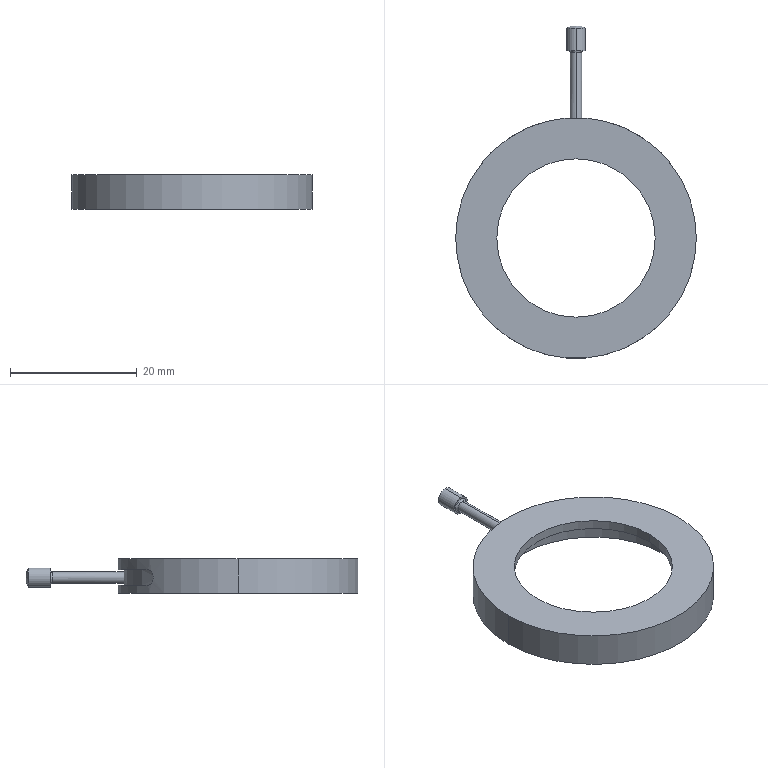Part | SolidWorks | features BaseBody 2 | 2 solids | 33 faces | box 38 x 52.6 x 5.5 mm | volume 2350 mm3 | cylinder 17 | plane 9 | spline 5 | cone 2 | commonest cylinder face diameters 1.6 x4 1 x2 1.8 x2 3 x2 25 x2 31.6 x2
STEP:
#1=CARTESIAN_POINT('',(12.618,14.205,1.7));
#2=VERTEX_POINT('',#1);
#3=CARTESIAN_POINT('',(-12.618,14.205,1.7));
#4=VERTEX_POINT('',#3);
#5=CARTESIAN_POINT('',(0.,0.,1.7));
#6=DIRECTION('',(0.,0.,1.));
#7=DIRECTION('',(-1.,0.,0.));
#8=AXIS2_PLACEMENT_3D('',#5,#6,#7);
#9=CIRCLE('',#8,19.);
#10=EDGE_CURVE('',#2,#4,#9,.T.);
#11=ORIENTED_EDGE('',*,*,#10,.T.);
#12=CARTESIAN_POINT('',(-12.618,14.205,-0.7));
#13=VERTEX_POINT('',#12);
#14=CARTESIAN_POINT('',(-12.618,14.205,1.7));
#15=CARTESIAN_POINT('',(-12.737,14.1,1.7));
#16=CARTESIAN_POINT('',(-12.852,13.995,1.669));
#17=CARTESIAN_POINT('',(-13.064,13.797,1.548));
#18=CARTESIAN_POINT('',(-13.16,13.705,1.459));
#19=CARTESIAN_POINT('',(-13.319,13.55,1.238));
#20=CARTESIAN_POINT('',(-13.383,13.487,1.104));
#21=CARTESIAN_POINT('',(-13.467,13.403,0.815));
#22=CARTESIAN_POINT('',(-13.49,13.38,0.657));
#23=CARTESIAN_POINT('',(-13.49,13.38,0.3439));
#24=CARTESIAN_POINT('',(-13.468,13.402,0.1866));
#25=CARTESIAN_POINT('',(-13.383,13.487,-0.1038));
#26=CARTESIAN_POINT('',(-13.32,13.549,-0.2361));
#27=CARTESIAN_POINT('',(-13.16,13.705,-0.4599));
#28=CARTESIAN_POINT('',(-13.065,13.796,-0.5481));
#29=CARTESIAN_POINT('',(-12.852,13.995,-0.6687));
#30=CARTESIAN_POINT('',(-12.737,14.1,-0.6996));
#31=CARTESIAN_POINT('',(-12.618,14.205,-0.7));
#32=B_SPLINE_CURVE_WITH_KNOTS('',3,(#14,#15,#16,#17,#18,#19,#20,#21,#22,#23,#24,#25,#26,#27,#28,#29,#30,#31),.UNSPECIFIED.,.F.,.F.,(4,2,2,2,2,2,2,2,4),(0.,0.0004687,0.0009374,0.001406,0.001875,0.002343,0.002812,0.003281,0.00375),.UNSPECIFIED.);
#33=EDGE_CURVE('',#4,#13,#32,.T.);
#34=ORIENTED_EDGE('',*,*,#33,.T.);
#35=CARTESIAN_POINT('',(12.618,14.205,-0.7));
#36=VERTEX_POINT('',#35);
#37=CARTESIAN_POINT('',(0.,0.,-0.7));
#38=DIRECTION('',(0.,0.,-1.));
#39=DIRECTION('',(-1.,0.,0.));
#40=AXIS2_PLACEMENT_3D('',#37,#38,#39);
#41=CIRCLE('',#40,19.);
#42=EDGE_CURVE('',#13,#36,#41,.T.);
#43=ORIENTED_EDGE('',*,*,#42,.T.);
#44=CARTESIAN_POINT('',(12.618,14.205,-0.7));
#45=CARTESIAN_POINT('',(12.737,14.1,-0.6996));
#46=CARTESIAN_POINT('',(12.852,13.995,-0.6689));
#47=CARTESIAN_POINT('',(13.064,13.797,-0.5484));
#48=CARTESIAN_POINT('',(13.16,13.705,-0.4594));
#49=CARTESIAN_POINT('',(13.319,13.55,-0.2378));
#50=CARTESIAN_POINT('',(13.383,13.487,-0.1039));
#51=CARTESIAN_POINT('',(13.467,13.403,0.185));
#52=CARTESIAN_POINT('',(13.49,13.38,0.343));
#53=CARTESIAN_POINT('',(13.49,13.38,0.6561));
#54=CARTESIAN_POINT('',(13.468,13.402,0.8134));
#55=CARTESIAN_POINT('',(13.383,13.487,1.104));
#56=CARTESIAN_POINT('',(13.32,13.549,1.236));
#57=CARTESIAN_POINT('',(13.16,13.705,1.46));
#58=CARTESIAN_POINT('',(13.065,13.796,1.548));
#59=CARTESIAN_POINT('',(12.852,13.995,1.669));
#60=CARTESIAN_POINT('',(12.737,14.1,1.7));
#61=CARTESIAN_POINT('',(12.618,14.205,1.7));
#62=B_SPLINE_CURVE_WITH_KNOTS('',3,(#44,#45,#46,#47,#48,#49,#50,#51,#52,#53,#54,#55,#56,#57,#58,#59,#60,#61),.UNSPECIFIED.,.F.,.F.,(4,2,2,2,2,2,2,2,4),(0.,0.0004687,0.0009374,0.001406,0.001875,0.002343,0.002812,0.003281,0.00375),.UNSPECIFIED.);
#63=EDGE_CURVE('',#36,#2,#62,.T.);
#64=ORIENTED_EDGE('',*,*,#63,.T.);
#65=EDGE_LOOP('',(#11,#34,#43,#64));
#66=FACE_BOUND('',#65,.T.);
#67=CARTESIAN_POINT('',(19.,0.,3.5));
#68=VERTEX_POINT('',#67);
#69=CARTESIAN_POINT('',(-19.,0.,3.5));
#70=VERTEX_POINT('',#69);
#71=CARTESIAN_POINT('',(0.,0.,3.5));
#72=DIRECTION('',(0.,0.,1.));
#73=DIRECTION('',(-1.,0.,0.));
#74=AXIS2_PLACEMENT_3D('',#71,#72,#73);
#75=CIRCLE('',#74,19.);
#76=EDGE_CURVE('',#68,#70,#75,.T.);
#77=ORIENTED_EDGE('',*,*,#76,.F.);
#78=CARTESIAN_POINT('',(19.,0.,-2.));
#79=VERTEX_POINT('',#78);
#80=CARTESIAN_POINT('',(19.,0.,3.5));
#81=DIRECTION('',(0.,0.,-1.));
#82=VECTOR('',#81,1000.);
#83=LINE('',#80,#82);
#84=EDGE_CURVE('',#68,#79,#83,.T.);
#85=ORIENTED_EDGE('',*,*,#84,.T.);
#86=CARTESIAN_POINT('',(-19.,0.,-2.));
#87=VERTEX_POINT('',#86);
#88=CARTESIAN_POINT('',(0.,0.,-2.));
#89=DIRECTION('',(0.,0.,1.));
#90=DIRECTION('',(-1.,0.,0.));
#91=AXIS2_PLACEMENT_3D('',#88,#89,#90);
#92=CIRCLE('',#91,19.);
#93=EDGE_CURVE('',#79,#87,#92,.T.);
#94=ORIENTED_EDGE('',*,*,#93,.T.);
#95=CARTESIAN_POINT('',(-19.,0.,3.5));
#96=DIRECTION('',(0.,0.,-1.));
#97=VECTOR('',#96,1000.);
#98=LINE('',#95,#97);
#99=EDGE_CURVE('',#70,#87,#98,.T.);
#100=ORIENTED_EDGE('',*,*,#99,.F.);
#101=EDGE_LOOP('',(#77,#85,#94,#100));
#102=FACE_OUTER_BOUND('',#101,.T.);
#103=CARTESIAN_POINT('',(0.,0.,3.5));
#104=DIRECTION('',(0.,0.,-1.));
#105=DIRECTION('',(-1.,0.,0.));
#106=AXIS2_PLACEMENT_3D('',#103,#104,#105);
#107=CYLINDRICAL_SURFACE('',#106,19.);
#108=ADVANCED_FACE('',(#66,#102),#107,.T.);
#109=CARTESIAN_POINT('',(-12.5,0.,2.));
#110=VERTEX_POINT('',#109);
#111=CARTESIAN_POINT('',(12.5,0.,2.));
#112=VERTEX_POINT('',#111);
#113=CARTESIAN_POINT('',(0.,0.,2.));
#114=DIRECTION('',(0.,0.,1.));
#115=DIRECTION('',(1.,0.,0.));
#116=AXIS2_PLACEMENT_3D('',#113,#114,#115);
#117=CIRCLE('',#116,12.5);
#118=EDGE_CURVE('',#110,#112,#117,.T.);
#119=ORIENTED_EDGE('',*,*,#118,.F.);
#120=CARTESIAN_POINT('',(-12.5,0.,3.5));
#121=VERTEX_POINT('',#120);
#122=CARTESIAN_POINT('',(-12.5,0.,-2.));
#123=DIRECTION('',(0.,0.,1.));
#124=VECTOR('',#123,1000.);
#125=LINE('',#122,#124);
#126=EDGE_CURVE('',#110,#121,#125,.T.);
#127=ORIENTED_EDGE('',*,*,#126,.T.);
#128=CARTESIAN_POINT('',(12.5,0.,3.5));
#129=VERTEX_POINT('',#128);
#130=CARTESIAN_POINT('',(0.,0.,3.5));
#131=DIRECTION('',(0.,0.,-1.));
#132=DIRECTION('',(1.,0.,0.));
#133=AXIS2_PLACEMENT_3D('',#130,#131,#132);
#134=CIRCLE('',#133,12.5);
#135=EDGE_CURVE('',#129,#121,#134,.T.);
#136=ORIENTED_EDGE('',*,*,#135,.F.);
#137=CARTESIAN_POINT('',(12.5,0.,-2.));
#138=DIRECTION('',(0.,0.,1.));
#139=VECTOR('',#138,1000.);
#140=LINE('',#137,#139);
#141=EDGE_CURVE('',#112,#129,#140,.T.);
#142=ORIENTED_EDGE('',*,*,#141,.F.);
#143=EDGE_LOOP('',(#119,#127,#136,#142));
#144=FACE_OUTER_BOUND('',#143,.T.);
#145=CARTESIAN_POINT('',(0.,0.,-2.));
#146=DIRECTION('',(0.,0.,1.));
#147=DIRECTION('',(1.,0.,0.));
#148=AXIS2_PLACEMENT_3D('',#145,#146,#147);
#149=CYLINDRICAL_SURFACE('',#148,12.5);
#150=ADVANCED_FACE('',(#144),#149,.F.);
#151=CARTESIAN_POINT('',(-15.8,0.,2.));
#152=VERTEX_POINT('',#151);
#153=CARTESIAN_POINT('',(15.8,0.,2.));
#154=VERTEX_POINT('',#153);
#155=CARTESIAN_POINT('',(0.,0.,2.));
#156=DIRECTION('',(0.,0.,1.));
#157=DIRECTION('',(-1.,0.,0.));
#158=AXIS2_PLACEMENT_3D('',#155,#156,#157);
#159=CIRCLE('',#158,15.8);
#160=EDGE_CURVE('',#152,#154,#159,.T.);
#161=ORIENTED_EDGE('',*,*,#160,.T.);
#162=CARTESIAN_POINT('',(15.8,0.,-2.));
#163=VERTEX_POINT('',#162);
#164=CARTESIAN_POINT('',(15.8,0.,2.));
#165=DIRECTION('',(0.,0.,-1.));
#166=VECTOR('',#165,1000.);
#167=LINE('',#164,#166);
#168=EDGE_CURVE('',#154,#163,#167,.T.);
#169=ORIENTED_EDGE('',*,*,#168,.T.);
#170=CARTESIAN_POINT('',(-15.8,0.,-2.));
#171=VERTEX_POINT('',#170);
#172=CARTESIAN_POINT('',(0.,0.,-2.));
#173=DIRECTION('',(0.,0.,-1.));
#174=DIRECTION('',(-1.,0.,0.));
#175=AXIS2_PLACEMENT_3D('',#172,#173,#174);
#176=CIRCLE('',#175,15.8);
#177=EDGE_CURVE('',#163,#171,#176,.T.);
#178=ORIENTED_EDGE('',*,*,#177,.T.);
#179=CARTESIAN_POINT('',(-15.8,0.,2.));
#180=DIRECTION('',(0.,0.,-1.));
#181=VECTOR('',#180,1000.);
#182=LINE('',#179,#181);
#183=EDGE_CURVE('',#152,#171,#182,.T.);
#184=ORIENTED_EDGE('',*,*,#183,.F.);
#185=EDGE_LOOP('',(#161,#169,#178,#184));
#186=FACE_OUTER_BOUND('',#185,.T.);
#187=CARTESIAN_POINT('',(0.,0.,2.));
#188=DIRECTION('',(0.,0.,-1.));
#189=DIRECTION('',(-1.,0.,0.));
#190=AXIS2_PLACEMENT_3D('',#187,#188,#189);
#191=CYLINDRICAL_SURFACE('',#190,15.8);
#192=ADVANCED_FACE('',(#186),#191,.F.);
#193=CARTESIAN_POINT('',(0.,18.,1.3));
#194=VERTEX_POINT('',#193);
#195=CARTESIAN_POINT('',(0.,18.,-0.3));
#196=VERTEX_POINT('',#195);
#197=CARTESIAN_POINT('',(0.,18.,1.3));
#198=CARTESIAN_POINT('',(-0.1057,18.,1.3));
#199=CARTESIAN_POINT('',(-0.2094,17.999,1.279));
#200=CARTESIAN_POINT('',(-0.4032,17.996,1.199));
#201=CARTESIAN_POINT('',(-0.4919,17.993,1.139));
#202=CARTESIAN_POINT('',(-0.7133,17.986,0.9181));
#203=CARTESIAN_POINT('',(-0.7999,17.982,0.7092));
#204=CARTESIAN_POINT('',(-0.8001,17.982,0.3962));
#205=CARTESIAN_POINT('',(-0.7794,17.983,0.2913));
#206=CARTESIAN_POINT('',(-0.6993,17.986,0.09761));
#207=CARTESIAN_POINT('',(-0.6407,17.989,0.009442));
#208=CARTESIAN_POINT('',(-0.4169,17.996,-0.2147));
#209=CARTESIAN_POINT('',(-0.2114,18.,-0.3));
#210=CARTESIAN_POINT('',(0.,18.,-0.3));
#211=B_SPLINE_CURVE_WITH_KNOTS('',3,(#197,#198,#199,#200,#201,#202,#203,#204,#205,#206,#207,#208,#209,#210),.UNSPECIFIED.,.F.,.F.,(4,2,2,2,2,2,4),(0.002501,0.002814,0.003126,0.003751,0.004064,0.004377,0.005002),.UNSPECIFIED.);
#212=EDGE_CURVE('',#194,#196,#211,.T.);
#213=ORIENTED_EDGE('',*,*,#212,.F.);
#214=CARTESIAN_POINT('',(0.,15.8,1.3));
#215=VERTEX_POINT('',#214);
#216=CARTESIAN_POINT('',(0.,37.5,1.3));
#217=DIRECTION('',(0.,-1.,0.));
#218=VECTOR('',#217,1000.);
#219=LINE('',#216,#218);
#220=EDGE_CURVE('',#194,#215,#219,.T.);
#221=ORIENTED_EDGE('',*,*,#220,.T.);
#222=CARTESIAN_POINT('',(0.,15.8,-0.3));
#223=VERTEX_POINT('',#222);
#224=CARTESIAN_POINT('',(0.,15.8,1.3));
#225=CARTESIAN_POINT('',(-0.1057,15.8,1.3));
#226=CARTESIAN_POINT('',(-0.2094,15.799,1.279));
#227=CARTESIAN_POINT('',(-0.4032,15.795,1.199));
#228=CARTESIAN_POINT('',(-0.4919,15.793,1.139));
#229=CARTESIAN_POINT('',(-0.7133,15.785,0.9181));
#230=CARTESIAN_POINT('',(-0.7999,15.78,0.7093));
#231=CARTESIAN_POINT('',(-0.8001,15.78,0.3962));
#232=CARTESIAN_POINT('',(-0.7794,15.781,0.2913));
#233=CARTESIAN_POINT('',(-0.6993,15.785,0.09761));
#234=CARTESIAN_POINT('',(-0.6407,15.787,0.009441));
#235=CARTESIAN_POINT('',(-0.4169,15.795,-0.2147));
#236=CARTESIAN_POINT('',(-0.2114,15.8,-0.3));
#237=CARTESIAN_POINT('',(0.,15.8,-0.3));
#238=B_SPLINE_CURVE_WITH_KNOTS('',3,(#224,#225,#226,#227,#228,#229,#230,#231,#232,#233,#234,#235,#236,#237),.UNSPECIFIED.,.F.,.F.,(4,2,2,2,2,2,4),(0.002501,0.002814,0.003126,0.003752,0.004064,0.004377,0.005002),.UNSPECIFIED.);
#239=EDGE_CURVE('',#215,#223,#238,.T.);
#240=ORIENTED_EDGE('',*,*,#239,.T.);
#241=CARTESIAN_POINT('',(0.,37.5,-0.3));
#242=DIRECTION('',(0.,-1.,0.));
#243=VECTOR('',#242,1000.);
#244=LINE('',#241,#243);
#245=EDGE_CURVE('',#196,#223,#244,.T.);
#246=ORIENTED_EDGE('',*,*,#245,.F.);
#247=EDGE_LOOP('',(#213,#221,#240,#246));
#248=FACE_OUTER_BOUND('',#247,.T.);
#249=CARTESIAN_POINT('',(0.,37.5,0.5));
#250=DIRECTION('',(0.,-1.,0.));
#251=DIRECTION('',(0.,0.,-1.));
#252=AXIS2_PLACEMENT_3D('',#249,#250,#251);
#253=CYLINDRICAL_SURFACE('',#252,0.8);
#254=ADVANCED_FACE('',(#248),#253,.F.);
#255=CARTESIAN_POINT('',(0.,0.,3.5));
#256=DIRECTION('',(0.,0.,1.));
#257=DIRECTION('',(-1.,0.,0.));
#258=AXIS2_PLACEMENT_3D('',#255,#256,#257);
#259=CIRCLE('',#258,19.);
#260=EDGE_CURVE('',#70,#68,#259,.T.);
#261=ORIENTED_EDGE('',*,*,#260,.T.);
#262=ORIENTED_EDGE('',*,*,#76,.T.);
#263=EDGE_LOOP('',(#261,#262));
#264=FACE_OUTER_BOUND('',#263,.T.);
#265=ORIENTED_EDGE('',*,*,#135,.T.);
#266=CARTESIAN_POINT('',(0.,0.,3.5));
#267=DIRECTION('',(0.,0.,-1.));
#268=DIRECTION('',(1.,0.,0.));
#269=AXIS2_PLACEMENT_3D('',#266,#267,#268);
#270=CIRCLE('',#269,12.5);
#271=EDGE_CURVE('',#121,#129,#270,.T.);
#272=ORIENTED_EDGE('',*,*,#271,.T.);
#273=EDGE_LOOP('',(#265,#272));
#274=FACE_BOUND('',#273,.T.);
#275=CARTESIAN_POINT('',(0.,0.,3.5));
#276=DIRECTION('',(0.,0.,1.));
#277=DIRECTION('',(1.,0.,0.));
#278=AXIS2_PLACEMENT_3D('',#275,#276,#277);
#279=PLANE('',#278);
#280=ADVANCED_FACE('',(#264,#274),#279,.T.);
#281=ORIENTED_EDGE('',*,*,#84,.F.);
#282=ORIENTED_EDGE('',*,*,#260,.F.);
#283=ORIENTED_EDGE('',*,*,#99,.T.);
#284=CARTESIAN_POINT('',(0.,0.,-2.));
#285=DIRECTION('',(0.,0.,1.));
#286=DIRECTION('',(-1.,0.,0.));
#287=AXIS2_PLACEMENT_3D('',#284,#285,#286);
#288=CIRCLE('',#287,19.);
#289=EDGE_CURVE('',#87,#79,#288,.T.);
#290=ORIENTED_EDGE('',*,*,#289,.T.);
#291=EDGE_LOOP('',(#281,#282,#283,#290));
#292=FACE_OUTER_BOUND('',#291,.T.);
#293=CARTESIAN_POINT('',(0.,0.,3.5));
#294=DIRECTION('',(0.,0.,-1.));
#295=DIRECTION('',(-1.,0.,0.));
#296=AXIS2_PLACEMENT_3D('',#293,#294,#295);
#297=CYLINDRICAL_SURFACE('',#296,19.);
#298=ADVANCED_FACE('',(#292),#297,.T.);
#299=ORIENTED_EDGE('',*,*,#126,.F.);
#300=CARTESIAN_POINT('',(0.,0.,2.));
#301=DIRECTION('',(0.,0.,1.));
#302=DIRECTION('',(1.,0.,0.));
#303=AXIS2_PLACEMENT_3D('',#300,#301,#302);
#304=CIRCLE('',#303,12.5);
#305=EDGE_CURVE('',#112,#110,#304,.T.);
#306=ORIENTED_EDGE('',*,*,#305,.F.);
#307=ORIENTED_EDGE('',*,*,#141,.T.);
#308=ORIENTED_EDGE('',*,*,#271,.F.);
#309=EDGE_LOOP('',(#299,#306,#307,#308));
#310=FACE_OUTER_BOUND('',#309,.T.);
#311=CARTESIAN_POINT('',(0.,0.,-2.));
#312=DIRECTION('',(0.,0.,1.));
#313=DIRECTION('',(1.,0.,0.));
#314=AXIS2_PLACEMENT_3D('',#311,#312,#313);
#315=CYLINDRICAL_SURFACE('',#314,12.5);
#316=ADVANCED_FACE('',(#310),#315,.F.);
#317=ORIENTED_EDGE('',*,*,#289,.F.);
#318=ORIENTED_EDGE('',*,*,#93,.F.);
#319=EDGE_LOOP('',(#317,#318));
#320=FACE_OUTER_BOUND('',#319,.T.);
#321=CARTESIAN_POINT('',(0.,0.,-2.));
#322=DIRECTION('',(0.,0.,-1.));
#323=DIRECTION('',(-1.,0.,0.));
#324=AXIS2_PLACEMENT_3D('',#321,#322,#323);
#325=CIRCLE('',#324,15.8);
#326=EDGE_CURVE('',#171,#163,#325,.T.);
#327=ORIENTED_EDGE('',*,*,#326,.F.);
#328=ORIENTED_EDGE('',*,*,#177,.F.);
#329=EDGE_LOOP('',(#327,#328));
#330=FACE_BOUND('',#329,.T.);
#331=CARTESIAN_POINT('',(0.,0.,-2.));
#332=DIRECTION('',(0.,0.,1.));
#333=DIRECTION('',(1.,0.,0.));
#334=AXIS2_PLACEMENT_3D('',#331,#332,#333);
#335=PLANE('',#334);
#336=ADVANCED_FACE('',(#320,#330),#335,.F.);
#337=ORIENTED_EDGE('',*,*,#33,.F.);
#338=CARTESIAN_POINT('',(-11.954,13.457,1.7));
#339=VERTEX_POINT('',#338);
#340=CARTESIAN_POINT('',(-12.286,13.831,1.7));
#341=DIRECTION('',(-0.6641,0.7476,0.));
#342=VECTOR('',#341,1000.);
#343=LINE('',#340,#342);
#344=EDGE_CURVE('',#339,#4,#343,.T.);
#345=ORIENTED_EDGE('',*,*,#344,.F.);
#346=CARTESIAN_POINT('',(-11.954,13.457,-0.7));
#347=VERTEX_POINT('',#346);
#348=CARTESIAN_POINT('',(-11.954,13.457,-0.7));
#349=CARTESIAN_POINT('',(-12.012,13.406,-0.6998));
#350=CARTESIAN_POINT('',(-12.068,13.355,-0.6919));
#351=CARTESIAN_POINT('',(-12.178,13.255,-0.6599));
#352=CARTESIAN_POINT('',(-12.233,13.205,-0.6353));
#353=CARTESIAN_POINT('',(-12.386,13.062,-0.5412));
#354=CARTESIAN_POINT('',(-12.477,12.974,-0.4487));
#355=CARTESIAN_POINT('',(-12.625,12.83,-0.2244));
#356=CARTESIAN_POINT('',(-12.683,12.773,-0.09072));
#357=CARTESIAN_POINT('',(-12.76,12.696,0.1945));
#358=CARTESIAN_POINT('',(-12.78,12.676,0.3479));
#359=CARTESIAN_POINT('',(-12.78,12.676,0.6537));
#360=CARTESIAN_POINT('',(-12.76,12.696,0.8061));
#361=CARTESIAN_POINT('',(-12.683,12.773,1.092));
#362=CARTESIAN_POINT('',(-12.626,12.83,1.224));
#363=CARTESIAN_POINT('',(-12.476,12.975,1.45));
#364=CARTESIAN_POINT('',(-12.386,13.061,1.541));
#365=CARTESIAN_POINT('',(-12.181,13.253,1.667));
#366=CARTESIAN_POINT('',(-12.07,13.355,1.7));
#367=CARTESIAN_POINT('',(-11.954,13.457,1.7));
#368=B_SPLINE_CURVE_WITH_KNOTS('',3,(#348,#349,#350,#351,#352,#353,#354,#355,#356,#357,#358,#359,#360,#361,#362,#363,#364,#365,#366,#367),.UNSPECIFIED.,.F.,.F.,(4,2,2,2,2,2,2,2,2,4),(0.,0.0002283,0.0004567,0.0009134,0.00137,0.001827,0.002283,0.00274,0.003197,0.003654),.UNSPECIFIED.);
#369=EDGE_CURVE('',#347,#339,#368,.T.);
#370=ORIENTED_EDGE('',*,*,#369,.F.);
#371=CARTESIAN_POINT('',(-12.286,13.831,-0.7));
#372=DIRECTION('',(0.6641,-0.7476,0.));
#373=VECTOR('',#372,1000.);
#374=LINE('',#371,#373);
#375=EDGE_CURVE('',#13,#347,#374,.T.);
#376=ORIENTED_EDGE('',*,*,#375,.F.);
#377=EDGE_LOOP('',(#337,#345,#370,#376));
#378=FACE_OUTER_BOUND('',#377,.T.);
#379=CARTESIAN_POINT('',(-12.625,14.212,-0.7));
#380=CARTESIAN_POINT('',(-12.745,14.106,-0.6996));
#381=CARTESIAN_POINT('',(-12.857,14.003,-0.6695));
#382=CARTESIAN_POINT('',(-13.072,13.803,-0.5478));
#383=CARTESIAN_POINT('',(-13.166,13.713,-0.461));
#384=CARTESIAN_POINT('',(-13.328,13.556,-0.236));
#385=CARTESIAN_POINT('',(-13.389,13.495,-0.1061));
#386=CARTESIAN_POINT('',(-13.475,13.409,0.1876));
#387=CARTESIAN_POINT('',(-13.497,13.387,0.341));
#388=CARTESIAN_POINT('',(-13.497,13.387,0.659));
#389=CARTESIAN_POINT('',(-13.475,13.409,0.8122));
#390=CARTESIAN_POINT('',(-13.389,13.495,1.106));
#391=CARTESIAN_POINT('',(-13.328,13.556,1.236));
#392=CARTESIAN_POINT('',(-13.166,13.713,1.461));
#393=CARTESIAN_POINT('',(-13.072,13.804,1.548));
#394=CARTESIAN_POINT('',(-12.858,14.003,1.669));
#395=CARTESIAN_POINT('',(-12.745,14.106,1.7));
#396=CARTESIAN_POINT('',(-12.625,14.212,1.7));
#397=CARTESIAN_POINT('',(-12.618,14.205,-0.7));
#398=CARTESIAN_POINT('',(-12.738,14.098,-0.6996));
#399=CARTESIAN_POINT('',(-12.85,13.996,-0.6695));
#400=CARTESIAN_POINT('',(-13.065,13.796,-0.5478));
#401=CARTESIAN_POINT('',(-13.159,13.706,-0.461));
#402=CARTESIAN_POINT('',(-13.321,13.549,-0.236));
#403=CARTESIAN_POINT('',(-13.382,13.488,-0.1061));
#404=CARTESIAN_POINT('',(-13.468,13.402,0.1876));
#405=CARTESIAN_POINT('',(-13.49,13.38,0.341));
#406=CARTESIAN_POINT('',(-13.49,13.38,0.659));
#407=CARTESIAN_POINT('',(-13.468,13.402,0.8122));
#408=CARTESIAN_POINT('',(-13.382,13.488,1.106));
#409=CARTESIAN_POINT('',(-13.321,13.549,1.236));
#410=CARTESIAN_POINT('',(-13.159,13.706,1.461));
#411=CARTESIAN_POINT('',(-13.065,13.796,1.548));
#412=CARTESIAN_POINT('',(-12.851,13.995,1.669));
#413=CARTESIAN_POINT('',(-12.738,14.099,1.7));
#414=CARTESIAN_POINT('',(-12.618,14.205,1.7));
#415=CARTESIAN_POINT('',(-11.954,13.457,-0.7));
#416=CARTESIAN_POINT('',(-12.068,13.356,-0.6996));
#417=CARTESIAN_POINT('',(-12.174,13.259,-0.6695));
#418=CARTESIAN_POINT('',(-12.378,13.069,-0.5478));
#419=CARTESIAN_POINT('',(-12.467,12.984,-0.461));
#420=CARTESIAN_POINT('',(-12.619,12.836,-0.236));
#421=CARTESIAN_POINT('',(-12.678,12.778,-0.1061));
#422=CARTESIAN_POINT('',(-12.759,12.697,0.1876));
#423=CARTESIAN_POINT('',(-12.78,12.676,0.341));
#424=CARTESIAN_POINT('',(-12.78,12.676,0.659));
#425=CARTESIAN_POINT('',(-12.759,12.696,0.8122));
#426=CARTESIAN_POINT('',(-12.678,12.778,1.106));
#427=CARTESIAN_POINT('',(-12.619,12.836,1.236));
#428=CARTESIAN_POINT('',(-12.467,12.984,1.461));
#429=CARTESIAN_POINT('',(-12.377,13.07,1.548));
#430=CARTESIAN_POINT('',(-12.175,13.259,1.669));
#431=CARTESIAN_POINT('',(-12.068,13.357,1.7));
#432=CARTESIAN_POINT('',(-11.954,13.457,1.7));
#433=CARTESIAN_POINT('',(-11.948,13.45,-0.7));
#434=CARTESIAN_POINT('',(-12.061,13.349,-0.6996));
#435=CARTESIAN_POINT('',(-12.167,13.252,-0.6695));
#436=CARTESIAN_POINT('',(-12.371,13.062,-0.5478));
#437=CARTESIAN_POINT('',(-12.46,12.977,-0.461));
#438=CARTESIAN_POINT('',(-12.612,12.829,-0.236));
#439=CARTESIAN_POINT('',(-12.671,12.771,-0.1061));
#440=CARTESIAN_POINT('',(-12.752,12.689,0.1876));
#441=CARTESIAN_POINT('',(-12.773,12.669,0.341));
#442=CARTESIAN_POINT('',(-12.773,12.669,0.659));
#443=CARTESIAN_POINT('',(-12.752,12.689,0.8122));
#444=CARTESIAN_POINT('',(-12.671,12.771,1.106));
#445=CARTESIAN_POINT('',(-12.612,12.829,1.236));
#446=CARTESIAN_POINT('',(-12.46,12.977,1.461));
#447=CARTESIAN_POINT('',(-12.37,13.063,1.548));
#448=CARTESIAN_POINT('',(-12.168,13.251,1.669));
#449=CARTESIAN_POINT('',(-12.061,13.349,1.7));
#450=CARTESIAN_POINT('',(-11.948,13.45,1.7));
#451=B_SPLINE_SURFACE_WITH_KNOTS('',1,3,((#379,#380,#381,#382,#383,#384,#385,#386,#387,#388,#389,#390,#391,#392,#393,#394,#395,#396),(#397,#398,#399,#400,#401,#402,#403,#404,#405,#406,#407,#408,#409,#410,#411,#412,#413,#414),(#415,#416,#417,#418,#419,#420,#421,#422,#423,#424,#425,#426,#427,#428,#429,#430,#431,#432),(#433,#434,#435,#436,#437,#438,#439,#440,#441,#442,#443,#444,#445,#446,#447,#448,#449,#450)),.UNSPECIFIED.,.F.,.F.,.F.,(2,1,1,2),(4,2,2,2,2,2,2,2,4),(-0.0101,0.,1.,1.01),(0.,0.125,0.25,0.375,0.5,0.625,0.75,0.875,1.),.UNSPECIFIED.);
#452=ADVANCED_FACE('',(#378),#451,.F.);
#453=ORIENTED_EDGE('',*,*,#344,.T.);
#454=ORIENTED_EDGE('',*,*,#10,.F.);
#455=CARTESIAN_POINT('',(11.954,13.457,1.7));
#456=VERTEX_POINT('',#455);
#457=CARTESIAN_POINT('',(11.954,13.457,1.7));
#458=DIRECTION('',(0.6641,0.7476,0.));
#459=VECTOR('',#458,1000.);
#460=LINE('',#457,#459);
#461=EDGE_CURVE('',#456,#2,#460,.T.);
#462=ORIENTED_EDGE('',*,*,#461,.F.);
#463=CARTESIAN_POINT('',(0.,0.,1.7));
#464=DIRECTION('',(0.,0.,-1.));
#465=DIRECTION('',(-1.,0.,0.));
#466=AXIS2_PLACEMENT_3D('',#463,#464,#465);
#467=CIRCLE('',#466,18.);
#468=EDGE_CURVE('',#339,#456,#467,.T.);
#469=ORIENTED_EDGE('',*,*,#468,.F.);
#470=EDGE_LOOP('',(#453,#454,#462,#469));
#471=FACE_OUTER_BOUND('',#470,.T.);
#472=CARTESIAN_POINT('',(0.,0.,1.7));
#473=DIRECTION('',(0.,0.,1.));
#474=DIRECTION('',(1.,0.,0.));
#475=AXIS2_PLACEMENT_3D('',#472,#473,#474);
#476=PLANE('',#475);
#477=ADVANCED_FACE('',(#471),#476,.F.);
#478=ORIENTED_EDGE('',*,*,#63,.F.);
#479=CARTESIAN_POINT('',(11.954,13.457,-0.7));
#480=VERTEX_POINT('',#479);
#481=CARTESIAN_POINT('',(12.286,13.831,-0.7));
#482=DIRECTION('',(0.6641,0.7476,0.));
#483=VECTOR('',#482,1000.);
#484=LINE('',#481,#483);
#485=EDGE_CURVE('',#480,#36,#484,.T.);
#486=ORIENTED_EDGE('',*,*,#485,.F.);
#487=CARTESIAN_POINT('',(11.954,13.457,1.7));
#488=CARTESIAN_POINT('',(12.012,13.406,1.7));
#489=CARTESIAN_POINT('',(12.068,13.355,1.692));
#490=CARTESIAN_POINT('',(12.178,13.255,1.66));
#491=CARTESIAN_POINT('',(12.233,13.205,1.635));
#492=CARTESIAN_POINT('',(12.386,13.062,1.541));
#493=CARTESIAN_POINT('',(12.477,12.974,1.449));
#494=CARTESIAN_POINT('',(12.625,12.83,1.224));
#495=CARTESIAN_POINT('',(12.683,12.773,1.091));
#496=CARTESIAN_POINT('',(12.76,12.696,0.8055));
#497=CARTESIAN_POINT('',(12.78,12.676,0.6521));
#498=CARTESIAN_POINT('',(12.78,12.676,0.3463));
#499=CARTESIAN_POINT('',(12.76,12.696,0.1939));
#500=CARTESIAN_POINT('',(12.683,12.773,-0.09225));
#501=CARTESIAN_POINT('',(12.626,12.83,-0.2237));
#502=CARTESIAN_POINT('',(12.476,12.975,-0.4498));
#503=CARTESIAN_POINT('',(12.386,13.061,-0.5408));
#504=CARTESIAN_POINT('',(12.181,13.253,-0.667));
#505=CARTESIAN_POINT('',(12.07,13.355,-0.6996));
#506=CARTESIAN_POINT('',(11.954,13.457,-0.7));
#507=B_SPLINE_CURVE_WITH_KNOTS('',3,(#487,#488,#489,#490,#491,#492,#493,#494,#495,#496,#497,#498,#499,#500,#501,#502,#503,#504,#505,#506),.UNSPECIFIED.,.F.,.F.,(4,2,2,2,2,2,2,2,2,4),(0.,0.0002283,0.0004567,0.0009134,0.00137,0.001827,0.002283,0.00274,0.003197,0.003654),.UNSPECIFIED.);
#508=EDGE_CURVE('',#456,#480,#507,.T.);
#509=ORIENTED_EDGE('',*,*,#508,.F.);
#510=ORIENTED_EDGE('',*,*,#461,.T.);
#511=EDGE_LOOP('',(#478,#486,#509,#510));
#512=FACE_OUTER_BOUND('',#511,.T.);
#513=CARTESIAN_POINT('',(12.625,14.212,1.7));
#514=CARTESIAN_POINT('',(12.745,14.106,1.7));
#515=CARTESIAN_POINT('',(12.857,14.003,1.67));
#516=CARTESIAN_POINT('',(13.072,13.803,1.548));
#517=CARTESIAN_POINT('',(13.166,13.713,1.461));
#518=CARTESIAN_POINT('',(13.328,13.556,1.236));
#519=CARTESIAN_POINT('',(13.389,13.495,1.106));
#520=CARTESIAN_POINT('',(13.475,13.409,0.8124));
#521=CARTESIAN_POINT('',(13.497,13.387,0.659));
#522=CARTESIAN_POINT('',(13.497,13.387,0.341));
#523=CARTESIAN_POINT('',(13.475,13.409,0.1878));
#524=CARTESIAN_POINT('',(13.389,13.495,-0.1062));
#525=CARTESIAN_POINT('',(13.328,13.556,-0.236));
#526=CARTESIAN_POINT('',(13.166,13.713,-0.461));
#527=CARTESIAN_POINT('',(13.072,13.804,-0.5481));
#528=CARTESIAN_POINT('',(12.858,14.003,-0.6692));
#529=CARTESIAN_POINT('',(12.745,14.106,-0.6996));
#530=CARTESIAN_POINT('',(12.625,14.212,-0.7));
#531=CARTESIAN_POINT('',(12.618,14.205,1.7));
#532=CARTESIAN_POINT('',(12.738,14.098,1.7));
#533=CARTESIAN_POINT('',(12.85,13.996,1.67));
#534=CARTESIAN_POINT('',(13.065,13.796,1.548));
#535=CARTESIAN_POINT('',(13.159,13.706,1.461));
#536=CARTESIAN_POINT('',(13.321,13.549,1.236));
#537=CARTESIAN_POINT('',(13.382,13.488,1.106));
#538=CARTESIAN_POINT('',(13.468,13.402,0.8124));
#539=CARTESIAN_POINT('',(13.49,13.38,0.659));
#540=CARTESIAN_POINT('',(13.49,13.38,0.341));
#541=CARTESIAN_POINT('',(13.468,13.402,0.1878));
#542=CARTESIAN_POINT('',(13.382,13.488,-0.1062));
#543=CARTESIAN_POINT('',(13.321,13.549,-0.236));
#544=CARTESIAN_POINT('',(13.159,13.706,-0.461));
#545=CARTESIAN_POINT('',(13.065,13.796,-0.5481));
#546=CARTESIAN_POINT('',(12.851,13.995,-0.6692));
#547=CARTESIAN_POINT('',(12.738,14.099,-0.6996));
#548=CARTESIAN_POINT('',(12.618,14.205,-0.7));
#549=CARTESIAN_POINT('',(11.954,13.457,1.7));
#550=CARTESIAN_POINT('',(12.068,13.356,1.7));
#551=CARTESIAN_POINT('',(12.174,13.259,1.67));
#552=CARTESIAN_POINT('',(12.378,13.069,1.548));
#553=CARTESIAN_POINT('',(12.467,12.984,1.461));
#554=CARTESIAN_POINT('',(12.619,12.836,1.236));
#555=CARTESIAN_POINT('',(12.678,12.778,1.106));
#556=CARTESIAN_POINT('',(12.759,12.697,0.8124));
#557=CARTESIAN_POINT('',(12.78,12.676,0.659));
#558=CARTESIAN_POINT('',(12.78,12.676,0.341));
#559=CARTESIAN_POINT('',(12.759,12.696,0.1878));
#560=CARTESIAN_POINT('',(12.678,12.778,-0.1062));
#561=CARTESIAN_POINT('',(12.619,12.836,-0.236));
#562=CARTESIAN_POINT('',(12.467,12.984,-0.461));
#563=CARTESIAN_POINT('',(12.377,13.07,-0.5481));
#564=CARTESIAN_POINT('',(12.175,13.259,-0.6692));
#565=CARTESIAN_POINT('',(12.068,13.357,-0.6996));
#566=CARTESIAN_POINT('',(11.954,13.457,-0.7));
#567=CARTESIAN_POINT('',(11.948,13.45,1.7));
#568=CARTESIAN_POINT('',(12.061,13.349,1.7));
#569=CARTESIAN_POINT('',(12.167,13.252,1.67));
#570=CARTESIAN_POINT('',(12.371,13.062,1.548));
#571=CARTESIAN_POINT('',(12.46,12.977,1.461));
#572=CARTESIAN_POINT('',(12.612,12.829,1.236));
#573=CARTESIAN_POINT('',(12.671,12.771,1.106));
#574=CARTESIAN_POINT('',(12.752,12.689,0.8124));
#575=CARTESIAN_POINT('',(12.773,12.669,0.659));
#576=CARTESIAN_POINT('',(12.773,12.669,0.341));
#577=CARTESIAN_POINT('',(12.752,12.689,0.1878));
#578=CARTESIAN_POINT('',(12.671,12.771,-0.1062));
#579=CARTESIAN_POINT('',(12.612,12.829,-0.236));
#580=CARTESIAN_POINT('',(12.46,12.977,-0.461));
#581=CARTESIAN_POINT('',(12.37,13.063,-0.5481));
#582=CARTESIAN_POINT('',(12.168,13.251,-0.6692));
#583=CARTESIAN_POINT('',(12.061,13.349,-0.6996));
#584=CARTESIAN_POINT('',(11.948,13.45,-0.7));
#585=B_SPLINE_SURFACE_WITH_KNOTS('',1,3,((#513,#514,#515,#516,#517,#518,#519,#520,#521,#522,#523,#524,#525,#526,#527,#528,#529,#530),(#531,#532,#533,#534,#535,#536,#537,#538,#539,#540,#541,#542,#543,#544,#545,#546,#547,#548),(#549,#550,#551,#552,#553,#554,#555,#556,#557,#558,#559,#560,#561,#562,#563,#564,#565,#566),(#567,#568,#569,#570,#571,#572,#573,#574,#575,#576,#577,#578,#579,#580,#581,#582,#583,#584)),.UNSPECIFIED.,.F.,.F.,.F.,(2,1,1,2),(4,2,2,2,2,2,2,2,4),(-0.0101,0.,1.,1.01),(0.,0.125,0.25,0.375,0.5,0.625,0.75,0.875,1.),.UNSPECIFIED.);
#586=ADVANCED_FACE('',(#512),#585,.F.);
#587=ORIENTED_EDGE('',*,*,#375,.T.);
#588=CARTESIAN_POINT('',(0.,0.,-0.7));
#589=DIRECTION('',(0.,0.,-1.));
#590=DIRECTION('',(-1.,0.,0.));
#591=AXIS2_PLACEMENT_3D('',#588,#589,#590);
#592=CIRCLE('',#591,18.);
#593=EDGE_CURVE('',#347,#480,#592,.T.);
#594=ORIENTED_EDGE('',*,*,#593,.T.);
#595=ORIENTED_EDGE('',*,*,#485,.T.);
#596=ORIENTED_EDGE('',*,*,#42,.F.);
#597=EDGE_LOOP('',(#587,#594,#595,#596));
#598=FACE_OUTER_BOUND('',#597,.T.);
#599=CARTESIAN_POINT('',(0.,0.,-0.7));
#600=DIRECTION('',(0.,0.,1.));
#601=DIRECTION('',(1.,0.,0.));
#602=AXIS2_PLACEMENT_3D('',#599,#600,#601);
#603=PLANE('',#602);
#604=ADVANCED_FACE('',(#598),#603,.T.);
#605=ORIENTED_EDGE('',*,*,#160,.F.);
#606=CARTESIAN_POINT('',(0.,0.,2.));
#607=DIRECTION('',(0.,0.,1.));
#608=DIRECTION('',(-1.,0.,0.));
#609=AXIS2_PLACEMENT_3D('',#606,#607,#608);
#610=CIRCLE('',#609,15.8);
#611=EDGE_CURVE('',#154,#152,#610,.T.);
#612=ORIENTED_EDGE('',*,*,#611,.F.);
#613=EDGE_LOOP('',(#605,#612));
#614=FACE_OUTER_BOUND('',#613,.T.);
#615=ORIENTED_EDGE('',*,*,#305,.T.);
#616=ORIENTED_EDGE('',*,*,#118,.T.);
#617=EDGE_LOOP('',(#615,#616));
#618=FACE_BOUND('',#617,.T.);
#619=CARTESIAN_POINT('',(0.,0.,2.));
#620=DIRECTION('',(0.,0.,1.));
#621=DIRECTION('',(1.,0.,0.));
#622=AXIS2_PLACEMENT_3D('',#619,#620,#621);
#623=PLANE('',#622);
#624=ADVANCED_FACE('',(#614,#618),#623,.F.);
#625=ORIENTED_EDGE('',*,*,#168,.F.);
#626=ORIENTED_EDGE('',*,*,#611,.T.);
#627=ORIENTED_EDGE('',*,*,#183,.T.);
#628=ORIENTED_EDGE('',*,*,#326,.T.);
#629=EDGE_LOOP('',(#625,#626,#627,#628));
#630=FACE_OUTER_BOUND('',#629,.T.);
#631=CARTESIAN_POINT('',(0.,15.8,-0.3));
#632=CARTESIAN_POINT('',(0.1057,15.8,-0.3));
#633=CARTESIAN_POINT('',(0.2094,15.799,-0.2792));
#634=CARTESIAN_POINT('',(0.4032,15.795,-0.1989));
#635=CARTESIAN_POINT('',(0.4919,15.793,-0.1395));
#636=CARTESIAN_POINT('',(0.7133,15.785,0.0819));
#637=CARTESIAN_POINT('',(0.7999,15.78,0.2907));
#638=CARTESIAN_POINT('',(0.8001,15.78,0.6038));
#639=CARTESIAN_POINT('',(0.7794,15.781,0.7087));
#640=CARTESIAN_POINT('',(0.6993,15.785,0.9024));
#641=CARTESIAN_POINT('',(0.6407,15.787,0.9906));
#642=CARTESIAN_POINT('',(0.4169,15.795,1.215));
#643=CARTESIAN_POINT('',(0.2114,15.8,1.3));
#644=CARTESIAN_POINT('',(0.,15.8,1.3));
#645=B_SPLINE_CURVE_WITH_KNOTS('',3,(#631,#632,#633,#634,#635,#636,#637,#638,#639,#640,#641,#642,#643,#644),.UNSPECIFIED.,.F.,.F.,(4,2,2,2,2,2,4),(0.,0.0003126,0.0006253,0.001251,0.001563,0.001876,0.002501),.UNSPECIFIED.);
#646=EDGE_CURVE('',#223,#215,#645,.T.);
#647=ORIENTED_EDGE('',*,*,#646,.F.);
#648=ORIENTED_EDGE('',*,*,#239,.F.);
#649=EDGE_LOOP('',(#647,#648));
#650=FACE_BOUND('',#649,.T.);
#651=CARTESIAN_POINT('',(0.,0.,2.));
#652=DIRECTION('',(0.,0.,-1.));
#653=DIRECTION('',(-1.,0.,0.));
#654=AXIS2_PLACEMENT_3D('',#651,#652,#653);
#655=CYLINDRICAL_SURFACE('',#654,15.8);
#656=ADVANCED_FACE('',(#630,#650),#655,.F.);
#657=ORIENTED_EDGE('',*,*,#508,.T.);
#658=ORIENTED_EDGE('',*,*,#593,.F.);
#659=ORIENTED_EDGE('',*,*,#369,.T.);
#660=ORIENTED_EDGE('',*,*,#468,.T.);
#661=EDGE_LOOP('',(#657,#658,#659,#660));
#662=FACE_OUTER_BOUND('',#661,.T.);
#663=CARTESIAN_POINT('',(0.,18.,-0.3));
#664=CARTESIAN_POINT('',(0.1057,18.,-0.3));
#665=CARTESIAN_POINT('',(0.2094,17.999,-0.2792));
#666=CARTESIAN_POINT('',(0.4032,17.996,-0.1989));
#667=CARTESIAN_POINT('',(0.4919,17.993,-0.1395));
#668=CARTESIAN_POINT('',(0.7133,17.986,0.08191));
#669=CARTESIAN_POINT('',(0.7999,17.982,0.2908));
#670=CARTESIAN_POINT('',(0.8001,17.982,0.6038));
#671=CARTESIAN_POINT('',(0.7794,17.983,0.7087));
#672=CARTESIAN_POINT('',(0.6993,17.986,0.9024));
#673=CARTESIAN_POINT('',(0.6407,17.989,0.9906));
#674=CARTESIAN_POINT('',(0.4169,17.996,1.215));
#675=CARTESIAN_POINT('',(0.2114,18.,1.3));
#676=CARTESIAN_POINT('',(0.,18.,1.3));
#677=B_SPLINE_CURVE_WITH_KNOTS('',3,(#663,#664,#665,#666,#667,#668,#669,#670,#671,#672,#673,#674,#675,#676),.UNSPECIFIED.,.F.,.F.,(4,2,2,2,2,2,4),(0.,0.0003126,0.0006252,0.00125,0.001563,0.001876,0.002501),.UNSPECIFIED.);
#678=EDGE_CURVE('',#196,#194,#677,.T.);
#679=ORIENTED_EDGE('',*,*,#678,.T.);
#680=ORIENTED_EDGE('',*,*,#212,.T.);
#681=EDGE_LOOP('',(#679,#680));
#682=FACE_BOUND('',#681,.T.);
#683=CARTESIAN_POINT('',(0.,0.,3.5));
#684=DIRECTION('',(0.,0.,-1.));
#685=DIRECTION('',(-1.,0.,0.));
#686=AXIS2_PLACEMENT_3D('',#683,#684,#685);
#687=CYLINDRICAL_SURFACE('',#686,18.);
#688=ADVANCED_FACE('',(#662,#682),#687,.T.);
#689=ORIENTED_EDGE('',*,*,#220,.F.);
#690=ORIENTED_EDGE('',*,*,#678,.F.);
#691=ORIENTED_EDGE('',*,*,#245,.T.);
#692=ORIENTED_EDGE('',*,*,#646,.T.);
#693=EDGE_LOOP('',(#689,#690,#691,#692));
#694=FACE_OUTER_BOUND('',#693,.T.);
#695=CARTESIAN_POINT('',(0.,37.5,0.5));
#696=DIRECTION('',(0.,-1.,0.));
#697=DIRECTION('',(0.,0.,-1.));
#698=AXIS2_PLACEMENT_3D('',#695,#696,#697);
#699=CYLINDRICAL_SURFACE('',#698,0.8);
#700=ADVANCED_FACE('',(#694),#699,.F.);
#701=CLOSED_SHELL('',(#108,#150,#192,#254,#280,#298,#316,#336,#452,#477,#586,#604,#624,#656,#688,#700));
#702=MANIFOLD_SOLID_BREP('',#701);
#703=CARTESIAN_POINT('',(-0.6563,29.6,1.505));
#704=VERTEX_POINT('',#703);
#705=CARTESIAN_POINT('',(0.6563,29.6,-0.5046));
#706=VERTEX_POINT('',#705);
#707=CARTESIAN_POINT('',(-0.6563,29.6,1.505));
#708=CARTESIAN_POINT('',(-0.5925,29.6,1.546));
#709=CARTESIAN_POINT('',(-0.4927,29.6,1.599));
#710=CARTESIAN_POINT('',(-0.369,29.6,1.643));
#711=CARTESIAN_POINT('',(-0.3144,29.6,1.658));
#712=CARTESIAN_POINT('',(-0.2777,29.6,1.668));
#713=CARTESIAN_POINT('',(-0.2607,29.6,1.672));
#714=CARTESIAN_POINT('',(-0.0785,29.6,1.709));
#715=CARTESIAN_POINT('',(0.08443,29.6,1.708));
#716=CARTESIAN_POINT('',(0.3272,29.6,1.658));
#717=CARTESIAN_POINT('',(0.4436,29.6,1.621));
#718=CARTESIAN_POINT('',(0.5709,29.6,1.557));
#719=CARTESIAN_POINT('',(0.6236,29.6,1.525));
#720=CARTESIAN_POINT('',(0.6584,29.6,1.503));
#721=CARTESIAN_POINT('',(0.6769,29.6,1.491));
#722=CARTESIAN_POINT('',(0.8169,29.6,1.392));
#723=CARTESIAN_POINT('',(0.9213,29.6,1.284));
#724=CARTESIAN_POINT('',(1.046,29.6,1.093));
#725=CARTESIAN_POINT('',(1.099,29.6,0.9929));
#726=CARTESIAN_POINT('',(1.143,29.6,0.8691));
#727=CARTESIAN_POINT('',(1.158,29.6,0.8145));
#728=CARTESIAN_POINT('',(1.168,29.6,0.7777));
#729=CARTESIAN_POINT('',(1.172,29.6,0.7607));
#730=CARTESIAN_POINT('',(1.209,29.6,0.5785));
#731=CARTESIAN_POINT('',(1.208,29.6,0.4156));
#732=CARTESIAN_POINT('',(1.158,29.6,0.1728));
#733=CARTESIAN_POINT('',(1.121,29.6,0.05636));
#734=CARTESIAN_POINT('',(1.057,29.6,-0.07092));
#735=CARTESIAN_POINT('',(1.025,29.6,-0.1236));
#736=CARTESIAN_POINT('',(1.003,29.6,-0.1584));
#737=CARTESIAN_POINT('',(0.991,29.6,-0.1769));
#738=CARTESIAN_POINT('',(0.8921,29.6,-0.317));
#739=CARTESIAN_POINT('',(0.7842,29.6,-0.421));
#740=CARTESIAN_POINT('',(0.6563,29.6,-0.5046));
#741=B_SPLINE_CURVE_WITH_KNOTS('',3,(#707,#708,#709,#710,#711,#712,#713,#714,#715,#716,#717,#718,#719,#720,#721,#722,#723,#724,#725,#726,#727,#728,#729,#730,#731,#732,#733,#734,#735,#736,#737,#738,#739,#740),.UNSPECIFIED.,.F.,.F.,(4,1,1,2,2,2,1,1,2,2,2,1,1,2,2,2,1,1,2,2,4),(0.,0.0625,0.09375,0.1094,0.125,0.25,0.3125,0.3437,0.3594,0.375,0.5,0.5625,0.5938,0.6094,0.625,0.75,0.8125,0.8438,0.8594,0.875,1.),.UNSPECIFIED.);
#742=EDGE_CURVE('',#704,#706,#741,.T.);
#743=ORIENTED_EDGE('',*,*,#742,.F.);
#744=CARTESIAN_POINT('',(-0.4922,29.3,1.253));
#745=VERTEX_POINT('',#744);
#746=CARTESIAN_POINT('',(-0.6563,29.3,1.505));
#747=DIRECTION('',(-0.8372,0.,-0.5469));
#748=DIRECTION('',(-0.5469,0.,0.8372));
#749=AXIS2_PLACEMENT_3D('',#746,#747,#748);
#750=CIRCLE('',#749,0.3);
#751=EDGE_CURVE('',#704,#745,#750,.T.);
#752=ORIENTED_EDGE('',*,*,#751,.T.);
#753=CARTESIAN_POINT('',(0.,29.3,1.4));
#754=VERTEX_POINT('',#753);
#755=CARTESIAN_POINT('',(0.,29.3,0.5));
#756=DIRECTION('',(0.,-1.,0.));
#757=DIRECTION('',(0.,0.,-1.));
#758=AXIS2_PLACEMENT_3D('',#755,#756,#757);
#759=CIRCLE('',#758,0.9);
#760=EDGE_CURVE('',#754,#745,#759,.T.);
#761=ORIENTED_EDGE('',*,*,#760,.F.);
#762=CARTESIAN_POINT('',(0.4922,29.3,-0.2535));
#763=VERTEX_POINT('',#762);
#764=CARTESIAN_POINT('',(0.,29.3,0.5));
#765=DIRECTION('',(0.,-1.,0.));
#766=DIRECTION('',(0.,0.,-1.));
#767=AXIS2_PLACEMENT_3D('',#764,#765,#766);
#768=CIRCLE('',#767,0.9);
#769=EDGE_CURVE('',#763,#754,#768,.T.);
#770=ORIENTED_EDGE('',*,*,#769,.F.);
#771=CARTESIAN_POINT('',(0.6563,29.3,-0.5046));
#772=DIRECTION('',(0.8372,0.,0.5469));
#773=DIRECTION('',(0.5469,0.,-0.8372));
#774=AXIS2_PLACEMENT_3D('',#771,#772,#773);
#775=CIRCLE('',#774,0.3);
#776=EDGE_CURVE('',#706,#763,#775,.T.);
#777=ORIENTED_EDGE('',*,*,#776,.F.);
#778=EDGE_LOOP('',(#743,#752,#761,#770,#777));
#779=FACE_OUTER_BOUND('',#778,.T.);
#780=CARTESIAN_POINT('',(0.6563,29.6,-0.5046));
#781=CARTESIAN_POINT('',(2.666,29.6,0.8081));
#782=CARTESIAN_POINT('',(1.353,29.6,2.817));
#783=CARTESIAN_POINT('',(-0.6563,29.6,1.505));
#784=CARTESIAN_POINT('',(0.5602,29.6,-0.3575));
#785=CARTESIAN_POINT('',(2.275,29.6,0.7629));
#786=CARTESIAN_POINT('',(1.155,29.6,2.478));
#787=CARTESIAN_POINT('',(-0.5602,29.6,1.357));
#788=CARTESIAN_POINT('',(0.4922,29.476,-0.2535));
#789=CARTESIAN_POINT('',(1.999,29.476,0.731));
#790=CARTESIAN_POINT('',(1.015,29.476,2.238));
#791=CARTESIAN_POINT('',(-0.4922,29.476,1.253));
#792=CARTESIAN_POINT('',(0.4922,29.3,-0.2535));
#793=CARTESIAN_POINT('',(1.999,29.3,0.731));
#794=CARTESIAN_POINT('',(1.015,29.3,2.238));
#795=CARTESIAN_POINT('',(-0.4922,29.3,1.253));
#796=(BOUNDED_SURFACE()B_SPLINE_SURFACE(3,3,((#780,#781,#782,#783),(#784,#785,#786,#787),(#788,#789,#790,#791),(#792,#793,#794,#795)),.UNSPECIFIED.,.F.,.F.,.F.)B_SPLINE_SURFACE_WITH_KNOTS((4,4),(4,4),(0.,1.),(0.,1.),.UNSPECIFIED.)GEOMETRIC_REPRESENTATION_ITEM()RATIONAL_B_SPLINE_SURFACE(((1.,0.3333,0.3333,1.),(0.8047,0.2682,0.2682,0.8047),(0.8047,0.2682,0.2682,0.8047),(1.,0.3333,0.3333,1.)))REPRESENTATION_ITEM('')SURFACE());
#797=ADVANCED_FACE('',(#779),#796,.F.);
#798=CARTESIAN_POINT('',(0.,29.3,-0.4));
#799=VERTEX_POINT('',#798);
#800=CARTESIAN_POINT('',(0.,29.3,0.5));
#801=DIRECTION('',(0.,-1.,0.));
#802=DIRECTION('',(0.,0.,-1.));
#803=AXIS2_PLACEMENT_3D('',#800,#801,#802);
#804=CIRCLE('',#803,0.9);
#805=EDGE_CURVE('',#799,#763,#804,.T.);
#806=ORIENTED_EDGE('',*,*,#805,.T.);
#807=ORIENTED_EDGE('',*,*,#769,.T.);
#808=CARTESIAN_POINT('',(0.,18.,1.4));
#809=VERTEX_POINT('',#808);
#810=CARTESIAN_POINT('',(0.,15.8,1.4));
#811=DIRECTION('',(0.,-1.,0.));
#812=VECTOR('',#811,1000.);
#813=LINE('',#810,#812);
#814=EDGE_CURVE('',#754,#809,#813,.T.);
#815=ORIENTED_EDGE('',*,*,#814,.T.);
#816=CARTESIAN_POINT('',(0.,18.,-0.4));
#817=VERTEX_POINT('',#816);
#818=CARTESIAN_POINT('',(0.,18.,0.5));
#819=DIRECTION('',(0.,1.,0.));
#820=DIRECTION('',(0.,0.,-1.));
#821=AXIS2_PLACEMENT_3D('',#818,#819,#820);
#822=CIRCLE('',#821,0.9);
#823=EDGE_CURVE('',#809,#817,#822,.T.);
#824=ORIENTED_EDGE('',*,*,#823,.T.);
#825=CARTESIAN_POINT('',(0.,15.8,-0.4));
#826=DIRECTION('',(0.,-1.,0.));
#827=VECTOR('',#826,1000.);
#828=LINE('',#825,#827);
#829=EDGE_CURVE('',#799,#817,#828,.T.);
#830=ORIENTED_EDGE('',*,*,#829,.F.);
#831=EDGE_LOOP('',(#806,#807,#815,#824,#830));
#832=FACE_OUTER_BOUND('',#831,.T.);
#833=CARTESIAN_POINT('',(0.,15.8,0.5));
#834=DIRECTION('',(0.,-1.,0.));
#835=DIRECTION('',(0.,0.,-1.));
#836=AXIS2_PLACEMENT_3D('',#833,#834,#835);
#837=CYLINDRICAL_SURFACE('',#836,0.9);
#838=ADVANCED_FACE('',(#832),#837,.T.);
#839=CARTESIAN_POINT('',(0.,18.,1.));
#840=VERTEX_POINT('',#839);
#841=CARTESIAN_POINT('',(0.,18.,0.));
#842=VERTEX_POINT('',#841);
#843=CARTESIAN_POINT('',(0.,18.,0.5));
#844=DIRECTION('',(0.,1.,0.));
#845=DIRECTION('',(0.,0.,-1.));
#846=AXIS2_PLACEMENT_3D('',#843,#844,#845);
#847=CIRCLE('',#846,0.5);
#848=EDGE_CURVE('',#840,#842,#847,.T.);
#849=ORIENTED_EDGE('',*,*,#848,.F.);
#850=CARTESIAN_POINT('',(0.,17.2,1.));
#851=VERTEX_POINT('',#850);
#852=CARTESIAN_POINT('',(0.,15.8,1.));
#853=DIRECTION('',(0.,-1.,0.));
#854=VECTOR('',#853,1000.);
#855=LINE('',#852,#854);
#856=EDGE_CURVE('',#840,#851,#855,.T.);
#857=ORIENTED_EDGE('',*,*,#856,.T.);
#858=CARTESIAN_POINT('',(0.,17.2,0.));
#859=VERTEX_POINT('',#858);
#860=CARTESIAN_POINT('',(0.,17.2,0.5));
#861=DIRECTION('',(0.,1.,0.));
#862=DIRECTION('',(0.,0.,-1.));
#863=AXIS2_PLACEMENT_3D('',#860,#861,#862);
#864=CIRCLE('',#863,0.5);
#865=EDGE_CURVE('',#851,#859,#864,.T.);
#866=ORIENTED_EDGE('',*,*,#865,.T.);
#867=CARTESIAN_POINT('',(0.,15.8,0.));
#868=DIRECTION('',(0.,-1.,0.));
#869=VECTOR('',#868,1000.);
#870=LINE('',#867,#869);
#871=EDGE_CURVE('',#842,#859,#870,.T.);
#872=ORIENTED_EDGE('',*,*,#871,.F.);
#873=EDGE_LOOP('',(#849,#857,#866,#872));
#874=FACE_OUTER_BOUND('',#873,.T.);
#875=CARTESIAN_POINT('',(0.,15.8,0.5));
#876=DIRECTION('',(0.,-1.,0.));
#877=DIRECTION('',(0.,0.,-1.));
#878=AXIS2_PLACEMENT_3D('',#875,#876,#877);
#879=CYLINDRICAL_SURFACE('',#878,0.5);
#880=ADVANCED_FACE('',(#874),#879,.T.);
#881=CARTESIAN_POINT('',(0.,33.1,-1.));
#882=VERTEX_POINT('',#881);
#883=CARTESIAN_POINT('',(0.,33.1,2.));
#884=VERTEX_POINT('',#883);
#885=CARTESIAN_POINT('',(0.,33.1,0.5));
#886=DIRECTION('',(0.,-1.,0.));
#887=DIRECTION('',(0.,0.,-1.));
#888=AXIS2_PLACEMENT_3D('',#885,#886,#887);
#889=CIRCLE('',#888,1.5);
#890=EDGE_CURVE('',#882,#884,#889,.T.);
#891=ORIENTED_EDGE('',*,*,#890,.T.);
#892=CARTESIAN_POINT('',(0.,29.6,2.));
#893=VERTEX_POINT('',#892);
#894=CARTESIAN_POINT('',(0.,15.8,2.));
#895=DIRECTION('',(0.,-1.,0.));
#896=VECTOR('',#895,1000.);
#897=LINE('',#894,#896);
#898=EDGE_CURVE('',#884,#893,#897,.T.);
#899=ORIENTED_EDGE('',*,*,#898,.T.);
#900=CARTESIAN_POINT('',(0.,29.6,-1.));
#901=VERTEX_POINT('',#900);
#902=CARTESIAN_POINT('',(0.,29.6,0.5));
#903=DIRECTION('',(0.,-1.,0.));
#904=DIRECTION('',(0.,0.,-1.));
#905=AXIS2_PLACEMENT_3D('',#902,#903,#904);
#906=CIRCLE('',#905,1.5);
#907=EDGE_CURVE('',#901,#893,#906,.T.);
#908=ORIENTED_EDGE('',*,*,#907,.F.);
#909=CARTESIAN_POINT('',(0.,15.8,-1.));
#910=DIRECTION('',(0.,-1.,0.));
#911=VECTOR('',#910,1000.);
#912=LINE('',#909,#911);
#913=EDGE_CURVE('',#882,#901,#912,.T.);
#914=ORIENTED_EDGE('',*,*,#913,.F.);
#915=EDGE_LOOP('',(#891,#899,#908,#914));
#916=FACE_OUTER_BOUND('',#915,.T.);
#917=CARTESIAN_POINT('',(0.,15.8,0.5));
#918=DIRECTION('',(0.,-1.,0.));
#919=DIRECTION('',(0.,0.,-1.));
#920=AXIS2_PLACEMENT_3D('',#917,#918,#919);
#921=CYLINDRICAL_SURFACE('',#920,1.5);
#922=ADVANCED_FACE('',(#916),#921,.T.);
#923=CARTESIAN_POINT('',(0.,17.2,1.3));
#924=VERTEX_POINT('',#923);
#925=CARTESIAN_POINT('',(0.,17.2,-0.3));
#926=VERTEX_POINT('',#925);
#927=CARTESIAN_POINT('',(0.,17.2,0.5));
#928=DIRECTION('',(0.,1.,0.));
#929=DIRECTION('',(0.,0.,-1.));
#930=AXIS2_PLACEMENT_3D('',#927,#928,#929);
#931=CIRCLE('',#930,0.8);
#932=EDGE_CURVE('',#924,#926,#931,.T.);
#933=ORIENTED_EDGE('',*,*,#932,.F.);
#934=CARTESIAN_POINT('',(0.,16.,1.3));
#935=VERTEX_POINT('',#934);
#936=CARTESIAN_POINT('',(0.,15.8,1.3));
#937=DIRECTION('',(0.,-1.,0.));
#938=VECTOR('',#937,1000.);
#939=LINE('',#936,#938);
#940=EDGE_CURVE('',#924,#935,#939,.T.);
#941=ORIENTED_EDGE('',*,*,#940,.T.);
#942=CARTESIAN_POINT('',(0.,16.,-0.3));
#943=VERTEX_POINT('',#942);
#944=CARTESIAN_POINT('',(0.,16.,0.5));
#945=DIRECTION('',(0.,1.,0.));
#946=DIRECTION('',(0.,0.,-1.));
#947=AXIS2_PLACEMENT_3D('',#944,#945,#946);
#948=CIRCLE('',#947,0.8);
#949=EDGE_CURVE('',#935,#943,#948,.T.);
#950=ORIENTED_EDGE('',*,*,#949,.T.);
#951=CARTESIAN_POINT('',(0.,15.8,-0.3));
#952=DIRECTION('',(0.,-1.,0.));
#953=VECTOR('',#952,1000.);
#954=LINE('',#951,#953);
#955=EDGE_CURVE('',#926,#943,#954,.T.);
#956=ORIENTED_EDGE('',*,*,#955,.F.);
#957=EDGE_LOOP('',(#933,#941,#950,#956));
#958=FACE_OUTER_BOUND('',#957,.T.);
#959=CARTESIAN_POINT('',(0.,15.8,0.5));
#960=DIRECTION('',(0.,-1.,0.));
#961=DIRECTION('',(0.,0.,-1.));
#962=AXIS2_PLACEMENT_3D('',#959,#960,#961);
#963=CYLINDRICAL_SURFACE('',#962,0.8);
#964=ADVANCED_FACE('',(#958),#963,.T.);
#965=CARTESIAN_POINT('',(0.,15.8,1.1));
#966=VERTEX_POINT('',#965);
#967=CARTESIAN_POINT('',(0.,15.8,-0.1));
#968=VERTEX_POINT('',#967);
#969=CARTESIAN_POINT('',(0.,15.8,0.5));
#970=DIRECTION('',(0.,1.,0.));
#971=DIRECTION('',(0.,0.,1.));
#972=AXIS2_PLACEMENT_3D('',#969,#970,#971);
#973=CIRCLE('',#972,0.6);
#974=EDGE_CURVE('',#966,#968,#973,.T.);
#975=ORIENTED_EDGE('',*,*,#974,.T.);
#976=CARTESIAN_POINT('',(0.,16.,-0.3));
#977=DIRECTION('',(0.,0.7071,-0.7071));
#978=VECTOR('',#977,1000.);
#979=LINE('',#976,#978);
#980=EDGE_CURVE('',#968,#943,#979,.T.);
#981=ORIENTED_EDGE('',*,*,#980,.T.);
#982=ORIENTED_EDGE('',*,*,#949,.F.);
#983=CARTESIAN_POINT('',(0.,16.,1.3));
#984=DIRECTION('',(0.,0.7071,0.7071));
#985=VECTOR('',#984,1000.);
#986=LINE('',#983,#985);
#987=EDGE_CURVE('',#966,#935,#986,.T.);
#988=ORIENTED_EDGE('',*,*,#987,.F.);
#989=EDGE_LOOP('',(#975,#981,#982,#988));
#990=FACE_OUTER_BOUND('',#989,.T.);
#991=CARTESIAN_POINT('',(0.,16.,0.5));
#992=DIRECTION('',(0.,1.,0.));
#993=DIRECTION('',(0.,0.,1.));
#994=AXIS2_PLACEMENT_3D('',#991,#992,#993);
#995=CONICAL_SURFACE('',#994,0.8,0.7854);
#996=ADVANCED_FACE('',(#990),#995,.T.);
#997=ORIENTED_EDGE('',*,*,#814,.F.);
#998=ORIENTED_EDGE('',*,*,#760,.T.);
#999=CARTESIAN_POINT('',(0.,29.3,0.5));
#1000=DIRECTION('',(0.,-1.,0.));
#1001=DIRECTION('',(0.,0.,-1.));
#1002=AXIS2_PLACEMENT_3D('',#999,#1000,#1001);
#1003=CIRCLE('',#1002,0.9);
#1004=EDGE_CURVE('',#745,#799,#1003,.T.);
#1005=ORIENTED_EDGE('',*,*,#1004,.T.);
#1006=ORIENTED_EDGE('',*,*,#829,.T.);
#1007=CARTESIAN_POINT('',(0.,18.,0.5));
#1008=DIRECTION('',(0.,1.,0.));
#1009=DIRECTION('',(0.,0.,-1.));
#1010=AXIS2_PLACEMENT_3D('',#1007,#1008,#1009);
#1011=CIRCLE('',#1010,0.9);
#1012=EDGE_CURVE('',#817,#809,#1011,.T.);
#1013=ORIENTED_EDGE('',*,*,#1012,.T.);
#1014=EDGE_LOOP('',(#997,#998,#1005,#1006,#1013));
#1015=FACE_OUTER_BOUND('',#1014,.T.);
#1016=CARTESIAN_POINT('',(0.,15.8,0.5));
#1017=DIRECTION('',(0.,-1.,0.));
#1018=DIRECTION('',(0.,0.,-1.));
#1019=AXIS2_PLACEMENT_3D('',#1016,#1017,#1018);
#1020=CYLINDRICAL_SURFACE('',#1019,0.9);
#1021=ADVANCED_FACE('',(#1015),#1020,.T.);
#1022=ORIENTED_EDGE('',*,*,#1012,.F.);
#1023=ORIENTED_EDGE('',*,*,#823,.F.);
#1024=EDGE_LOOP('',(#1022,#1023));
#1025=FACE_OUTER_BOUND('',#1024,.T.);
#1026=CARTESIAN_POINT('',(0.,18.,0.5));
#1027=DIRECTION('',(0.,1.,0.));
#1028=DIRECTION('',(0.,0.,-1.));
#1029=AXIS2_PLACEMENT_3D('',#1026,#1027,#1028);
#1030=CIRCLE('',#1029,0.5);
#1031=EDGE_CURVE('',#842,#840,#1030,.T.);
#1032=ORIENTED_EDGE('',*,*,#1031,.T.);
#1033=ORIENTED_EDGE('',*,*,#848,.T.);
#1034=EDGE_LOOP('',(#1032,#1033));
#1035=FACE_BOUND('',#1034,.T.);
#1036=CARTESIAN_POINT('',(0.6697,18.,0.9376));
#1037=DIRECTION('',(0.,-1.,0.));
#1038=DIRECTION('',(0.,0.,-1.));
#1039=AXIS2_PLACEMENT_3D('',#1036,#1037,#1038);
#1040=PLANE('',#1039);
#1041=ADVANCED_FACE('',(#1025,#1035),#1040,.T.);
#1042=ORIENTED_EDGE('',*,*,#751,.F.);
#1043=CARTESIAN_POINT('',(0.6563,29.6,-0.5046));
#1044=CARTESIAN_POINT('',(0.5925,29.6,-0.5463));
#1045=CARTESIAN_POINT('',(0.4927,29.6,-0.5989));
#1046=CARTESIAN_POINT('',(0.369,29.6,-0.6431));
#1047=CARTESIAN_POINT('',(0.3144,29.6,-0.6583));
#1048=CARTESIAN_POINT('',(0.2777,29.6,-0.6676));
#1049=CARTESIAN_POINT('',(0.2607,29.6,-0.6715));
#1050=CARTESIAN_POINT('',(0.0785,29.6,-0.7089));
#1051=CARTESIAN_POINT('',(-0.08443,29.6,-0.7083));
#1052=CARTESIAN_POINT('',(-0.3272,29.6,-0.6575));
#1053=CARTESIAN_POINT('',(-0.4436,29.6,-0.6205));
#1054=CARTESIAN_POINT('',(-0.5709,29.6,-0.5571));
#1055=CARTESIAN_POINT('',(-0.6236,29.6,-0.5255));
#1056=CARTESIAN_POINT('',(-0.6584,29.6,-0.5035));
#1057=CARTESIAN_POINT('',(-0.6769,29.6,-0.491));
#1058=CARTESIAN_POINT('',(-0.8169,29.6,-0.3922));
#1059=CARTESIAN_POINT('',(-0.9213,29.6,-0.2838));
#1060=CARTESIAN_POINT('',(-1.046,29.6,-0.09262));
#1061=CARTESIAN_POINT('',(-1.099,29.6,0.007143));
#1062=CARTESIAN_POINT('',(-1.143,29.6,0.1309));
#1063=CARTESIAN_POINT('',(-1.158,29.6,0.1855));
#1064=CARTESIAN_POINT('',(-1.168,29.6,0.2223));
#1065=CARTESIAN_POINT('',(-1.172,29.6,0.2393));
#1066=CARTESIAN_POINT('',(-1.209,29.6,0.4215));
#1067=CARTESIAN_POINT('',(-1.208,29.6,0.5844));
#1068=CARTESIAN_POINT('',(-1.158,29.6,0.8272));
#1069=CARTESIAN_POINT('',(-1.121,29.6,0.9436));
#1070=CARTESIAN_POINT('',(-1.057,29.6,1.071));
#1071=CARTESIAN_POINT('',(-1.025,29.6,1.124));
#1072=CARTESIAN_POINT('',(-1.003,29.6,1.158));
#1073=CARTESIAN_POINT('',(-0.991,29.6,1.177));
#1074=CARTESIAN_POINT('',(-0.8921,29.6,1.317));
#1075=CARTESIAN_POINT('',(-0.7842,29.6,1.421));
#1076=CARTESIAN_POINT('',(-0.6563,29.6,1.505));
#1077=B_SPLINE_CURVE_WITH_KNOTS('',3,(#1043,#1044,#1045,#1046,#1047,#1048,#1049,#1050,#1051,#1052,#1053,#1054,#1055,#1056,#1057,#1058,#1059,#1060,#1061,#1062,#1063,#1064,#1065,#1066,#1067,#1068,#1069,#1070,#1071,#1072,#1073,#1074,#1075,#1076),.UNSPECIFIED.,.F.,.F.,(4,1,1,2,2,2,1,1,2,2,2,1,1,2,2,2,1,1,2,2,4),(0.,0.0625,0.09375,0.1094,0.125,0.25,0.3125,0.3437,0.3594,0.375,0.5,0.5625,0.5937,0.6094,0.625,0.75,0.8125,0.8437,0.8594,0.875,1.),.UNSPECIFIED.);
#1078=EDGE_CURVE('',#706,#704,#1077,.T.);
#1079=ORIENTED_EDGE('',*,*,#1078,.F.);
#1080=ORIENTED_EDGE('',*,*,#776,.T.);
#1081=ORIENTED_EDGE('',*,*,#805,.F.);
#1082=ORIENTED_EDGE('',*,*,#1004,.F.);
#1083=EDGE_LOOP('',(#1042,#1079,#1080,#1081,#1082));
#1084=FACE_OUTER_BOUND('',#1083,.T.);
#1085=CARTESIAN_POINT('',(-0.6563,29.6,1.505));
#1086=CARTESIAN_POINT('',(-2.666,29.6,0.1919));
#1087=CARTESIAN_POINT('',(-1.353,29.6,-1.817));
#1088=CARTESIAN_POINT('',(0.6563,29.6,-0.5046));
#1089=CARTESIAN_POINT('',(-0.5602,29.6,1.357));
#1090=CARTESIAN_POINT('',(-2.275,29.6,0.2371));
#1091=CARTESIAN_POINT('',(-1.155,29.6,-1.478));
#1092=CARTESIAN_POINT('',(0.5602,29.6,-0.3575));
#1093=CARTESIAN_POINT('',(-0.4922,29.476,1.253));
#1094=CARTESIAN_POINT('',(-1.999,29.476,0.269));
#1095=CARTESIAN_POINT('',(-1.015,29.476,-1.238));
#1096=CARTESIAN_POINT('',(0.4922,29.476,-0.2535));
#1097=CARTESIAN_POINT('',(-0.4922,29.3,1.253));
#1098=CARTESIAN_POINT('',(-1.999,29.3,0.269));
#1099=CARTESIAN_POINT('',(-1.015,29.3,-1.238));
#1100=CARTESIAN_POINT('',(0.4922,29.3,-0.2535));
#1101=(BOUNDED_SURFACE()B_SPLINE_SURFACE(3,3,((#1085,#1086,#1087,#1088),(#1089,#1090,#1091,#1092),(#1093,#1094,#1095,#1096),(#1097,#1098,#1099,#1100)),.UNSPECIFIED.,.F.,.F.,.F.)B_SPLINE_SURFACE_WITH_KNOTS((4,4),(4,4),(0.,1.),(0.,1.),.UNSPECIFIED.)GEOMETRIC_REPRESENTATION_ITEM()RATIONAL_B_SPLINE_SURFACE(((1.,0.3333,0.3333,1.),(0.8047,0.2682,0.2682,0.8047),(0.8047,0.2682,0.2682,0.8047),(1.,0.3333,0.3333,1.)))REPRESENTATION_ITEM('')SURFACE());
#1102=ADVANCED_FACE('',(#1084),#1101,.F.);
#1103=ORIENTED_EDGE('',*,*,#856,.F.);
#1104=ORIENTED_EDGE('',*,*,#1031,.F.);
#1105=ORIENTED_EDGE('',*,*,#871,.T.);
#1106=CARTESIAN_POINT('',(0.,17.2,0.5));
#1107=DIRECTION('',(0.,1.,0.));
#1108=DIRECTION('',(0.,0.,-1.));
#1109=AXIS2_PLACEMENT_3D('',#1106,#1107,#1108);
#1110=CIRCLE('',#1109,0.5);
#1111=EDGE_CURVE('',#859,#851,#1110,.T.);
#1112=ORIENTED_EDGE('',*,*,#1111,.T.);
#1113=EDGE_LOOP('',(#1103,#1104,#1105,#1112));
#1114=FACE_OUTER_BOUND('',#1113,.T.);
#1115=CARTESIAN_POINT('',(0.,15.8,0.5));
#1116=DIRECTION('',(0.,-1.,0.));
#1117=DIRECTION('',(0.,0.,-1.));
#1118=AXIS2_PLACEMENT_3D('',#1115,#1116,#1117);
#1119=CYLINDRICAL_SURFACE('',#1118,0.5);
#1120=ADVANCED_FACE('',(#1114),#1119,.T.);
#1121=ORIENTED_EDGE('',*,*,#907,.T.);
#1122=CARTESIAN_POINT('',(0.,29.6,0.5));
#1123=DIRECTION('',(0.,-1.,0.));
#1124=DIRECTION('',(0.,0.,-1.));
#1125=AXIS2_PLACEMENT_3D('',#1122,#1123,#1124);
#1126=CIRCLE('',#1125,1.5);
#1127=EDGE_CURVE('',#893,#901,#1126,.T.);
#1128=ORIENTED_EDGE('',*,*,#1127,.T.);
#1129=EDGE_LOOP('',(#1121,#1128));
#1130=FACE_OUTER_BOUND('',#1129,.T.);
#1131=ORIENTED_EDGE('',*,*,#1078,.T.);
#1132=ORIENTED_EDGE('',*,*,#742,.T.);
#1133=EDGE_LOOP('',(#1131,#1132));
#1134=FACE_BOUND('',#1133,.T.);
#1135=CARTESIAN_POINT('',(0.7535,29.6,0.9922));
#1136=DIRECTION('',(0.,-1.,0.));
#1137=DIRECTION('',(0.,0.,-1.));
#1138=AXIS2_PLACEMENT_3D('',#1135,#1136,#1137);
#1139=PLANE('',#1138);
#1140=ADVANCED_FACE('',(#1130,#1134),#1139,.T.);
#1141=CARTESIAN_POINT('',(0.,17.2,0.5));
#1142=DIRECTION('',(0.,1.,0.));
#1143=DIRECTION('',(0.,0.,-1.));
#1144=AXIS2_PLACEMENT_3D('',#1141,#1142,#1143);
#1145=CIRCLE('',#1144,0.8);
#1146=EDGE_CURVE('',#926,#924,#1145,.T.);
#1147=ORIENTED_EDGE('',*,*,#1146,.T.);
#1148=ORIENTED_EDGE('',*,*,#932,.T.);
#1149=EDGE_LOOP('',(#1147,#1148));
#1150=FACE_OUTER_BOUND('',#1149,.T.);
#1151=ORIENTED_EDGE('',*,*,#1111,.F.);
#1152=ORIENTED_EDGE('',*,*,#865,.F.);
#1153=EDGE_LOOP('',(#1151,#1152));
#1154=FACE_BOUND('',#1153,.T.);
#1155=CARTESIAN_POINT('',(0.4186,17.2,0.7735));
#1156=DIRECTION('',(0.,1.,0.));
#1157=DIRECTION('',(0.,0.,1.));
#1158=AXIS2_PLACEMENT_3D('',#1155,#1156,#1157);
#1159=PLANE('',#1158);
#1160=ADVANCED_FACE('',(#1150,#1154),#1159,.T.);
#1161=ORIENTED_EDGE('',*,*,#898,.F.);
#1162=CARTESIAN_POINT('',(0.,33.1,0.5));
#1163=DIRECTION('',(0.,-1.,0.));
#1164=DIRECTION('',(0.,0.,-1.));
#1165=AXIS2_PLACEMENT_3D('',#1162,#1163,#1164);
#1166=CIRCLE('',#1165,1.5);
#1167=EDGE_CURVE('',#884,#882,#1166,.T.);
#1168=ORIENTED_EDGE('',*,*,#1167,.T.);
#1169=ORIENTED_EDGE('',*,*,#913,.T.);
#1170=ORIENTED_EDGE('',*,*,#1127,.F.);
#1171=EDGE_LOOP('',(#1161,#1168,#1169,#1170));
#1172=FACE_OUTER_BOUND('',#1171,.T.);
#1173=CARTESIAN_POINT('',(0.,15.8,0.5));
#1174=DIRECTION('',(0.,-1.,0.));
#1175=DIRECTION('',(0.,0.,-1.));
#1176=AXIS2_PLACEMENT_3D('',#1173,#1174,#1175);
#1177=CYLINDRICAL_SURFACE('',#1176,1.5);
#1178=ADVANCED_FACE('',(#1172),#1177,.T.);
#1179=ORIENTED_EDGE('',*,*,#940,.F.);
#1180=ORIENTED_EDGE('',*,*,#1146,.F.);
#1181=ORIENTED_EDGE('',*,*,#955,.T.);
#1182=CARTESIAN_POINT('',(0.,16.,0.5));
#1183=DIRECTION('',(0.,1.,0.));
#1184=DIRECTION('',(0.,0.,-1.));
#1185=AXIS2_PLACEMENT_3D('',#1182,#1183,#1184);
#1186=CIRCLE('',#1185,0.8);
#1187=EDGE_CURVE('',#943,#935,#1186,.T.);
#1188=ORIENTED_EDGE('',*,*,#1187,.T.);
#1189=EDGE_LOOP('',(#1179,#1180,#1181,#1188));
#1190=FACE_OUTER_BOUND('',#1189,.T.);
#1191=CARTESIAN_POINT('',(0.,15.8,0.5));
#1192=DIRECTION('',(0.,-1.,0.));
#1193=DIRECTION('',(0.,0.,-1.));
#1194=AXIS2_PLACEMENT_3D('',#1191,#1192,#1193);
#1195=CYLINDRICAL_SURFACE('',#1194,0.8);
#1196=ADVANCED_FACE('',(#1190),#1195,.T.);
#1197=ORIENTED_EDGE('',*,*,#890,.F.);
#1198=ORIENTED_EDGE('',*,*,#1167,.F.);
#1199=EDGE_LOOP('',(#1197,#1198));
#1200=FACE_OUTER_BOUND('',#1199,.T.);
#1201=CARTESIAN_POINT('',(1.939,32.669,0.3268));
#1202=CARTESIAN_POINT('',(1.534,33.237,0.9459));
#1203=CARTESIAN_POINT('',(1.024,33.237,1.727));
#1204=CARTESIAN_POINT('',(0.6197,32.669,2.345));
#1205=CARTESIAN_POINT('',(1.396,33.242,-0.5539));
#1206=CARTESIAN_POINT('',(0.8435,34.018,0.2914));
#1207=CARTESIAN_POINT('',(0.1471,34.018,1.357));
#1208=CARTESIAN_POINT('',(-0.405,33.242,2.202));
#1209=CARTESIAN_POINT('',(0.4056,33.243,-1.201));
#1210=CARTESIAN_POINT('',(-0.1467,34.018,-0.3556));
#1211=CARTESIAN_POINT('',(-0.8432,34.018,0.7104));
#1212=CARTESIAN_POINT('',(-1.395,33.242,1.556));
#1213=CARTESIAN_POINT('',(-0.6191,32.67,-1.345));
#1214=CARTESIAN_POINT('',(-1.024,33.238,-0.7254));
#1215=CARTESIAN_POINT('',(-1.534,33.238,0.05554));
#1216=CARTESIAN_POINT('',(-1.938,32.669,0.6746));
#1217=(BOUNDED_SURFACE()B_SPLINE_SURFACE(3,3,((#1201,#1202,#1203,#1204),(#1205,#1206,#1207,#1208),(#1209,#1210,#1211,#1212),(#1213,#1214,#1215,#1216)),.UNSPECIFIED.,.F.,.F.,.F.)B_SPLINE_SURFACE_WITH_KNOTS((4,4),(4,4),(0.,1.),(0.,1.),.UNSPECIFIED.)GEOMETRIC_REPRESENTATION_ITEM()RATIONAL_B_SPLINE_SURFACE(((1.,0.8619,0.8619,1.),(0.861,0.7422,0.7422,0.861),(0.861,0.7422,0.7422,0.861),(1.,0.8619,0.8619,1.)))REPRESENTATION_ITEM('')SURFACE());
#1218=ADVANCED_FACE('',(#1200),#1217,.T.);
#1219=ORIENTED_EDGE('',*,*,#980,.F.);
#1220=CARTESIAN_POINT('',(0.,15.8,0.5));
#1221=DIRECTION('',(0.,1.,0.));
#1222=DIRECTION('',(0.,0.,1.));
#1223=AXIS2_PLACEMENT_3D('',#1220,#1221,#1222);
#1224=CIRCLE('',#1223,0.6);
#1225=EDGE_CURVE('',#968,#966,#1224,.T.);
#1226=ORIENTED_EDGE('',*,*,#1225,.T.);
#1227=ORIENTED_EDGE('',*,*,#987,.T.);
#1228=ORIENTED_EDGE('',*,*,#1187,.F.);
#1229=EDGE_LOOP('',(#1219,#1226,#1227,#1228));
#1230=FACE_OUTER_BOUND('',#1229,.T.);
#1231=CARTESIAN_POINT('',(0.,16.,0.5));
#1232=DIRECTION('',(0.,1.,0.));
#1233=DIRECTION('',(0.,0.,1.));
#1234=AXIS2_PLACEMENT_3D('',#1231,#1232,#1233);
#1235=CONICAL_SURFACE('',#1234,0.8,0.7854);
#1236=ADVANCED_FACE('',(#1230),#1235,.T.);
#1237=ORIENTED_EDGE('',*,*,#974,.F.);
#1238=ORIENTED_EDGE('',*,*,#1225,.F.);
#1239=EDGE_LOOP('',(#1237,#1238));
#1240=FACE_OUTER_BOUND('',#1239,.T.);
#1241=CARTESIAN_POINT('',(0.,15.8,0.5));
#1242=DIRECTION('',(0.,-1.,0.));
#1243=DIRECTION('',(0.,0.,-1.));
#1244=AXIS2_PLACEMENT_3D('',#1241,#1242,#1243);
#1245=PLANE('',#1244);
#1246=ADVANCED_FACE('',(#1240),#1245,.T.);
#1247=CLOSED_SHELL('',(#797,#838,#880,#922,#964,#996,#1021,#1041,#1102,#1120,#1140,#1160,#1178,#1196,#1218,#1236,#1246));
#1248=MANIFOLD_SOLID_BREP('',#1247);
#1249=CARTESIAN_POINT('',(0.,0.,0.));
#1250=DIRECTION('',(0.,0.,1.));
#1251=DIRECTION('',(1.,0.,0.));
#1252=AXIS2_PLACEMENT_3D('',#1249,#1250,#1251);
#1253=(LENGTH_UNIT()NAMED_UNIT(*)SI_UNIT(.MILLI.,.METRE.));
#1254=UNCERTAINTY_MEASURE_WITH_UNIT(LENGTH_MEASURE(0.00001),#1253,'','');
#1255=(NAMED_UNIT(*)PLANE_ANGLE_UNIT()SI_UNIT($,.RADIAN.));
#1256=(NAMED_UNIT(*)SI_UNIT($,.STERADIAN.)SOLID_ANGLE_UNIT());
#1257=(GEOMETRIC_REPRESENTATION_CONTEXT(3)GLOBAL_UNCERTAINTY_ASSIGNED_CONTEXT((#1254))GLOBAL_UNIT_ASSIGNED_CONTEXT((#1253,#1255,#1256))REPRESENTATION_CONTEXT('',''));
#1258=ADVANCED_BREP_SHAPE_REPRESENTATION('',(#702,#1248,#1252),#1257);